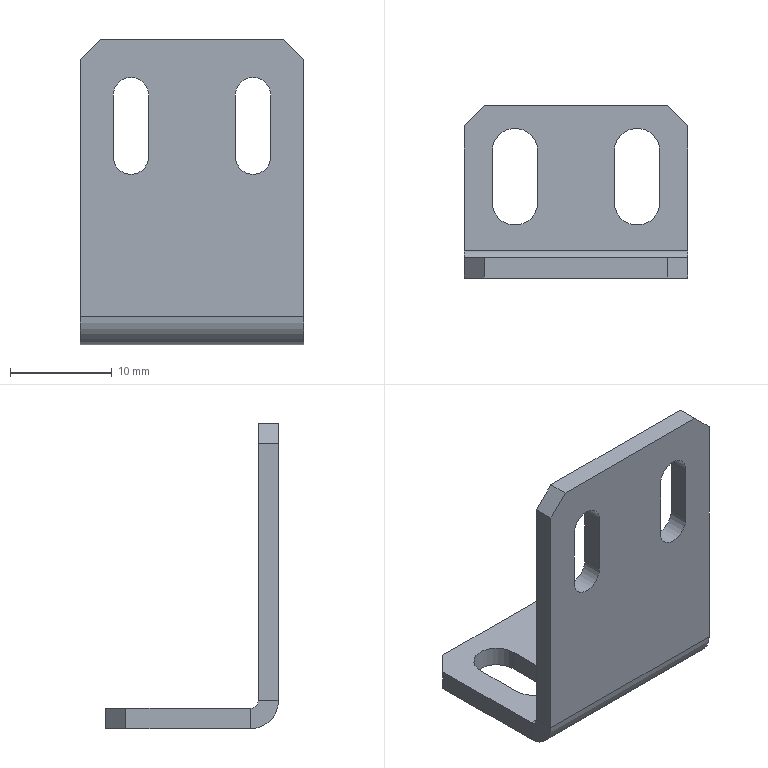Part | SolidWorks | features ICE 2, Chamfer 1, EdgeFlange 1, FlatPattern 1, SMBaseFlange 1, SheetMetal 1 | 1 solid | 36 faces | box 22 x 17 x 30 mm | volume 1655 mm3 | plane 24 | cylinder 12 | commonest cylinder face diameters 3.5 x6 4.5 x4 1.473 x1 5.473 x1
STEP:
#1=CARTESIAN_POINT('',(-6.,-2.,26.25));
#2=VERTEX_POINT('',#1);
#3=CARTESIAN_POINT('',(-4.25,-2.,24.5));
#4=VERTEX_POINT('',#3);
#5=CARTESIAN_POINT('',(-6.,-2.,24.5));
#6=DIRECTION('',(0.,1.,0.));
#7=DIRECTION('',(0.,0.,1.));
#8=AXIS2_PLACEMENT_3D('',#5,#6,#7);
#9=CIRCLE('',#8,1.75);
#10=EDGE_CURVE('',#2,#4,#9,.T.);
#11=ORIENTED_EDGE('',*,*,#10,.F.);
#12=CARTESIAN_POINT('',(-6.,0.,26.25));
#13=VERTEX_POINT('',#12);
#14=CARTESIAN_POINT('',(-6.,-10.,26.25));
#15=DIRECTION('',(0.,1.,0.));
#16=VECTOR('',#15,1000.);
#17=LINE('',#14,#16);
#18=EDGE_CURVE('',#2,#13,#17,.T.);
#19=ORIENTED_EDGE('',*,*,#18,.T.);
#20=CARTESIAN_POINT('',(-4.25,0.,24.5));
#21=VERTEX_POINT('',#20);
#22=CARTESIAN_POINT('',(-6.,0.,24.5));
#23=DIRECTION('',(0.,1.,0.));
#24=DIRECTION('',(0.,0.,1.));
#25=AXIS2_PLACEMENT_3D('',#22,#23,#24);
#26=CIRCLE('',#25,1.75);
#27=EDGE_CURVE('',#13,#21,#26,.T.);
#28=ORIENTED_EDGE('',*,*,#27,.T.);
#29=CARTESIAN_POINT('',(-4.25,-10.,24.5));
#30=DIRECTION('',(0.,1.,0.));
#31=VECTOR('',#30,1000.);
#32=LINE('',#29,#31);
#33=EDGE_CURVE('',#4,#21,#32,.T.);
#34=ORIENTED_EDGE('',*,*,#33,.F.);
#35=EDGE_LOOP('',(#11,#19,#28,#34));
#36=FACE_OUTER_BOUND('',#35,.T.);
#37=CARTESIAN_POINT('',(-6.,-10.,24.5));
#38=DIRECTION('',(0.,1.,0.));
#39=DIRECTION('',(0.,0.,1.));
#40=AXIS2_PLACEMENT_3D('',#37,#38,#39);
#41=CYLINDRICAL_SURFACE('',#40,1.75);
#42=ADVANCED_FACE('',(#36),#41,.F.);
#43=CARTESIAN_POINT('',(6.,-2.,26.25));
#44=VERTEX_POINT('',#43);
#45=CARTESIAN_POINT('',(7.75,-2.,24.5));
#46=VERTEX_POINT('',#45);
#47=CARTESIAN_POINT('',(6.,-2.,24.5));
#48=DIRECTION('',(0.,1.,0.));
#49=DIRECTION('',(0.,0.,1.));
#50=AXIS2_PLACEMENT_3D('',#47,#48,#49);
#51=CIRCLE('',#50,1.75);
#52=EDGE_CURVE('',#44,#46,#51,.T.);
#53=ORIENTED_EDGE('',*,*,#52,.F.);
#54=CARTESIAN_POINT('',(6.,0.,26.25));
#55=VERTEX_POINT('',#54);
#56=CARTESIAN_POINT('',(6.,-10.,26.25));
#57=DIRECTION('',(0.,1.,0.));
#58=VECTOR('',#57,1000.);
#59=LINE('',#56,#58);
#60=EDGE_CURVE('',#44,#55,#59,.T.);
#61=ORIENTED_EDGE('',*,*,#60,.T.);
#62=CARTESIAN_POINT('',(7.75,0.,24.5));
#63=VERTEX_POINT('',#62);
#64=CARTESIAN_POINT('',(6.,0.,24.5));
#65=DIRECTION('',(0.,1.,0.));
#66=DIRECTION('',(0.,0.,1.));
#67=AXIS2_PLACEMENT_3D('',#64,#65,#66);
#68=CIRCLE('',#67,1.75);
#69=EDGE_CURVE('',#55,#63,#68,.T.);
#70=ORIENTED_EDGE('',*,*,#69,.T.);
#71=CARTESIAN_POINT('',(7.75,-10.,24.5));
#72=DIRECTION('',(0.,1.,0.));
#73=VECTOR('',#72,1000.);
#74=LINE('',#71,#73);
#75=EDGE_CURVE('',#46,#63,#74,.T.);
#76=ORIENTED_EDGE('',*,*,#75,.F.);
#77=EDGE_LOOP('',(#53,#61,#70,#76));
#78=FACE_OUTER_BOUND('',#77,.T.);
#79=CARTESIAN_POINT('',(6.,-10.,24.5));
#80=DIRECTION('',(0.,1.,0.));
#81=DIRECTION('',(0.,0.,1.));
#82=AXIS2_PLACEMENT_3D('',#79,#80,#81);
#83=CYLINDRICAL_SURFACE('',#82,1.75);
#84=ADVANCED_FACE('',(#78),#83,.F.);
#85=CARTESIAN_POINT('',(-4.25,-2.,18.5));
#86=VERTEX_POINT('',#85);
#87=CARTESIAN_POINT('',(-4.25,-2.,30.));
#88=DIRECTION('',(0.,0.,-1.));
#89=VECTOR('',#88,1000.);
#90=LINE('',#87,#89);
#91=EDGE_CURVE('',#4,#86,#90,.T.);
#92=ORIENTED_EDGE('',*,*,#91,.T.);
#93=CARTESIAN_POINT('',(-7.75,-2.,18.5));
#94=VERTEX_POINT('',#93);
#95=CARTESIAN_POINT('',(-6.,-2.,18.5));
#96=DIRECTION('',(0.,1.,0.));
#97=DIRECTION('',(0.,0.,1.));
#98=AXIS2_PLACEMENT_3D('',#95,#96,#97);
#99=CIRCLE('',#98,1.75);
#100=EDGE_CURVE('',#86,#94,#99,.T.);
#101=ORIENTED_EDGE('',*,*,#100,.T.);
#102=CARTESIAN_POINT('',(-7.75,-2.,24.5));
#103=VERTEX_POINT('',#102);
#104=CARTESIAN_POINT('',(-7.75,-2.,30.));
#105=DIRECTION('',(0.,0.,1.));
#106=VECTOR('',#105,1000.);
#107=LINE('',#104,#106);
#108=EDGE_CURVE('',#94,#103,#107,.T.);
#109=ORIENTED_EDGE('',*,*,#108,.T.);
#110=CARTESIAN_POINT('',(-6.,-2.,24.5));
#111=DIRECTION('',(0.,1.,0.));
#112=DIRECTION('',(0.,0.,1.));
#113=AXIS2_PLACEMENT_3D('',#110,#111,#112);
#114=CIRCLE('',#113,1.75);
#115=EDGE_CURVE('',#103,#2,#114,.T.);
#116=ORIENTED_EDGE('',*,*,#115,.T.);
#117=ORIENTED_EDGE('',*,*,#10,.T.);
#118=EDGE_LOOP('',(#92,#101,#109,#116,#117));
#119=FACE_BOUND('',#118,.T.);
#120=CARTESIAN_POINT('',(7.75,-2.,18.5));
#121=VERTEX_POINT('',#120);
#122=CARTESIAN_POINT('',(7.75,-2.,30.));
#123=DIRECTION('',(0.,0.,-1.));
#124=VECTOR('',#123,1000.);
#125=LINE('',#122,#124);
#126=EDGE_CURVE('',#46,#121,#125,.T.);
#127=ORIENTED_EDGE('',*,*,#126,.T.);
#128=CARTESIAN_POINT('',(4.25,-2.,18.5));
#129=VERTEX_POINT('',#128);
#130=CARTESIAN_POINT('',(6.,-2.,18.5));
#131=DIRECTION('',(0.,1.,0.));
#132=DIRECTION('',(0.,0.,1.));
#133=AXIS2_PLACEMENT_3D('',#130,#131,#132);
#134=CIRCLE('',#133,1.75);
#135=EDGE_CURVE('',#121,#129,#134,.T.);
#136=ORIENTED_EDGE('',*,*,#135,.T.);
#137=CARTESIAN_POINT('',(4.25,-2.,24.5));
#138=VERTEX_POINT('',#137);
#139=CARTESIAN_POINT('',(4.25,-2.,30.));
#140=DIRECTION('',(0.,0.,1.));
#141=VECTOR('',#140,1000.);
#142=LINE('',#139,#141);
#143=EDGE_CURVE('',#129,#138,#142,.T.);
#144=ORIENTED_EDGE('',*,*,#143,.T.);
#145=CARTESIAN_POINT('',(6.,-2.,24.5));
#146=DIRECTION('',(0.,1.,0.));
#147=DIRECTION('',(0.,0.,1.));
#148=AXIS2_PLACEMENT_3D('',#145,#146,#147);
#149=CIRCLE('',#148,1.75);
#150=EDGE_CURVE('',#138,#44,#149,.T.);
#151=ORIENTED_EDGE('',*,*,#150,.T.);
#152=ORIENTED_EDGE('',*,*,#52,.T.);
#153=EDGE_LOOP('',(#127,#136,#144,#151,#152));
#154=FACE_BOUND('',#153,.T.);
#155=CARTESIAN_POINT('',(-9.,-2.,30.));
#156=VERTEX_POINT('',#155);
#157=CARTESIAN_POINT('',(9.,-2.,30.));
#158=VERTEX_POINT('',#157);
#159=CARTESIAN_POINT('',(-11.,-2.,30.));
#160=DIRECTION('',(1.,0.,0.));
#161=VECTOR('',#160,1000.);
#162=LINE('',#159,#161);
#163=EDGE_CURVE('',#156,#158,#162,.T.);
#164=ORIENTED_EDGE('',*,*,#163,.F.);
#165=CARTESIAN_POINT('',(-11.,-2.,28.));
#166=VERTEX_POINT('',#165);
#167=CARTESIAN_POINT('',(-11.,-2.,28.));
#168=DIRECTION('',(-0.7071,0.,-0.7071));
#169=VECTOR('',#168,1000.);
#170=LINE('',#167,#169);
#171=EDGE_CURVE('',#156,#166,#170,.T.);
#172=ORIENTED_EDGE('',*,*,#171,.T.);
#173=CARTESIAN_POINT('',(-11.,-2.,2.737));
#174=VERTEX_POINT('',#173);
#175=CARTESIAN_POINT('',(-11.,-2.,30.));
#176=DIRECTION('',(0.,0.,-1.));
#177=VECTOR('',#176,1000.);
#178=LINE('',#175,#177);
#179=EDGE_CURVE('',#166,#174,#178,.T.);
#180=ORIENTED_EDGE('',*,*,#179,.T.);
#181=CARTESIAN_POINT('',(11.,-2.,2.737));
#182=VERTEX_POINT('',#181);
#183=CARTESIAN_POINT('',(-11.,-2.,2.737));
#184=DIRECTION('',(1.,0.,0.));
#185=VECTOR('',#184,1000.);
#186=LINE('',#183,#185);
#187=EDGE_CURVE('',#174,#182,#186,.T.);
#188=ORIENTED_EDGE('',*,*,#187,.T.);
#189=CARTESIAN_POINT('',(11.,-2.,28.));
#190=VERTEX_POINT('',#189);
#191=CARTESIAN_POINT('',(11.,-2.,30.));
#192=DIRECTION('',(0.,0.,-1.));
#193=VECTOR('',#192,1000.);
#194=LINE('',#191,#193);
#195=EDGE_CURVE('',#190,#182,#194,.T.);
#196=ORIENTED_EDGE('',*,*,#195,.F.);
#197=CARTESIAN_POINT('',(11.,-2.,28.));
#198=DIRECTION('',(-0.7071,0.,0.7071));
#199=VECTOR('',#198,1000.);
#200=LINE('',#197,#199);
#201=EDGE_CURVE('',#190,#158,#200,.T.);
#202=ORIENTED_EDGE('',*,*,#201,.T.);
#203=EDGE_LOOP('',(#164,#172,#180,#188,#196,#202));
#204=FACE_OUTER_BOUND('',#203,.T.);
#205=CARTESIAN_POINT('',(-11.,-2.,30.));
#206=DIRECTION('',(0.,1.,0.));
#207=DIRECTION('',(0.,0.,1.));
#208=AXIS2_PLACEMENT_3D('',#205,#206,#207);
#209=PLANE('',#208);
#210=ADVANCED_FACE('',(#119,#154,#204),#209,.F.);
#211=CARTESIAN_POINT('',(-4.25,0.,18.5));
#212=VERTEX_POINT('',#211);
#213=CARTESIAN_POINT('',(-7.75,0.,18.5));
#214=VERTEX_POINT('',#213);
#215=CARTESIAN_POINT('',(-6.,0.,18.5));
#216=DIRECTION('',(0.,1.,0.));
#217=DIRECTION('',(0.,0.,1.));
#218=AXIS2_PLACEMENT_3D('',#215,#216,#217);
#219=CIRCLE('',#218,1.75);
#220=EDGE_CURVE('',#212,#214,#219,.T.);
#221=ORIENTED_EDGE('',*,*,#220,.F.);
#222=CARTESIAN_POINT('',(-4.25,0.,18.5));
#223=DIRECTION('',(0.,0.,-1.));
#224=VECTOR('',#223,1000.);
#225=LINE('',#222,#224);
#226=EDGE_CURVE('',#21,#212,#225,.T.);
#227=ORIENTED_EDGE('',*,*,#226,.F.);
#228=ORIENTED_EDGE('',*,*,#27,.F.);
#229=CARTESIAN_POINT('',(-7.75,0.,24.5));
#230=VERTEX_POINT('',#229);
#231=CARTESIAN_POINT('',(-6.,0.,24.5));
#232=DIRECTION('',(0.,1.,0.));
#233=DIRECTION('',(0.,0.,1.));
#234=AXIS2_PLACEMENT_3D('',#231,#232,#233);
#235=CIRCLE('',#234,1.75);
#236=EDGE_CURVE('',#230,#13,#235,.T.);
#237=ORIENTED_EDGE('',*,*,#236,.F.);
#238=CARTESIAN_POINT('',(-7.75,0.,18.5));
#239=DIRECTION('',(0.,0.,1.));
#240=VECTOR('',#239,1000.);
#241=LINE('',#238,#240);
#242=EDGE_CURVE('',#214,#230,#241,.T.);
#243=ORIENTED_EDGE('',*,*,#242,.F.);
#244=EDGE_LOOP('',(#221,#227,#228,#237,#243));
#245=FACE_BOUND('',#244,.T.);
#246=CARTESIAN_POINT('',(7.75,0.,18.5));
#247=VERTEX_POINT('',#246);
#248=CARTESIAN_POINT('',(4.25,0.,18.5));
#249=VERTEX_POINT('',#248);
#250=CARTESIAN_POINT('',(6.,0.,18.5));
#251=DIRECTION('',(0.,1.,0.));
#252=DIRECTION('',(0.,0.,1.));
#253=AXIS2_PLACEMENT_3D('',#250,#251,#252);
#254=CIRCLE('',#253,1.75);
#255=EDGE_CURVE('',#247,#249,#254,.T.);
#256=ORIENTED_EDGE('',*,*,#255,.F.);
#257=CARTESIAN_POINT('',(7.75,0.,18.5));
#258=DIRECTION('',(0.,0.,-1.));
#259=VECTOR('',#258,1000.);
#260=LINE('',#257,#259);
#261=EDGE_CURVE('',#63,#247,#260,.T.);
#262=ORIENTED_EDGE('',*,*,#261,.F.);
#263=ORIENTED_EDGE('',*,*,#69,.F.);
#264=CARTESIAN_POINT('',(4.25,0.,24.5));
#265=VERTEX_POINT('',#264);
#266=CARTESIAN_POINT('',(6.,0.,24.5));
#267=DIRECTION('',(0.,1.,0.));
#268=DIRECTION('',(0.,0.,1.));
#269=AXIS2_PLACEMENT_3D('',#266,#267,#268);
#270=CIRCLE('',#269,1.75);
#271=EDGE_CURVE('',#265,#55,#270,.T.);
#272=ORIENTED_EDGE('',*,*,#271,.F.);
#273=CARTESIAN_POINT('',(4.25,0.,18.5));
#274=DIRECTION('',(0.,0.,1.));
#275=VECTOR('',#274,1000.);
#276=LINE('',#273,#275);
#277=EDGE_CURVE('',#249,#265,#276,.T.);
#278=ORIENTED_EDGE('',*,*,#277,.F.);
#279=EDGE_LOOP('',(#256,#262,#263,#272,#278));
#280=FACE_BOUND('',#279,.T.);
#281=CARTESIAN_POINT('',(-11.,0.,28.));
#282=VERTEX_POINT('',#281);
#283=CARTESIAN_POINT('',(-11.,0.,2.737));
#284=VERTEX_POINT('',#283);
#285=CARTESIAN_POINT('',(-11.,0.,30.));
#286=DIRECTION('',(0.,0.,-1.));
#287=VECTOR('',#286,1000.);
#288=LINE('',#285,#287);
#289=EDGE_CURVE('',#282,#284,#288,.T.);
#290=ORIENTED_EDGE('',*,*,#289,.F.);
#291=CARTESIAN_POINT('',(-9.,0.,30.));
#292=VERTEX_POINT('',#291);
#293=CARTESIAN_POINT('',(-10.,0.,29.));
#294=DIRECTION('',(0.7071,0.,0.7071));
#295=VECTOR('',#294,1000.);
#296=LINE('',#293,#295);
#297=EDGE_CURVE('',#282,#292,#296,.T.);
#298=ORIENTED_EDGE('',*,*,#297,.T.);
#299=CARTESIAN_POINT('',(9.,0.,30.));
#300=VERTEX_POINT('',#299);
#301=CARTESIAN_POINT('',(-11.,0.,30.));
#302=DIRECTION('',(1.,0.,0.));
#303=VECTOR('',#302,1000.);
#304=LINE('',#301,#303);
#305=EDGE_CURVE('',#292,#300,#304,.T.);
#306=ORIENTED_EDGE('',*,*,#305,.T.);
#307=CARTESIAN_POINT('',(11.,0.,28.));
#308=VERTEX_POINT('',#307);
#309=CARTESIAN_POINT('',(-1.,0.,40.));
#310=DIRECTION('',(0.7071,0.,-0.7071));
#311=VECTOR('',#310,1000.);
#312=LINE('',#309,#311);
#313=EDGE_CURVE('',#300,#308,#312,.T.);
#314=ORIENTED_EDGE('',*,*,#313,.T.);
#315=CARTESIAN_POINT('',(11.,0.,2.737));
#316=VERTEX_POINT('',#315);
#317=CARTESIAN_POINT('',(11.,0.,30.));
#318=DIRECTION('',(0.,0.,-1.));
#319=VECTOR('',#318,1000.);
#320=LINE('',#317,#319);
#321=EDGE_CURVE('',#308,#316,#320,.T.);
#322=ORIENTED_EDGE('',*,*,#321,.T.);
#323=CARTESIAN_POINT('',(-11.,0.,2.737));
#324=DIRECTION('',(1.,0.,0.));
#325=VECTOR('',#324,1000.);
#326=LINE('',#323,#325);
#327=EDGE_CURVE('',#284,#316,#326,.T.);
#328=ORIENTED_EDGE('',*,*,#327,.F.);
#329=EDGE_LOOP('',(#290,#298,#306,#314,#322,#328));
#330=FACE_OUTER_BOUND('',#329,.T.);
#331=CARTESIAN_POINT('',(-11.,0.,30.));
#332=DIRECTION('',(0.,1.,0.));
#333=DIRECTION('',(0.,0.,1.));
#334=AXIS2_PLACEMENT_3D('',#331,#332,#333);
#335=PLANE('',#334);
#336=ADVANCED_FACE('',(#245,#280,#330),#335,.T.);
#337=ORIENTED_EDGE('',*,*,#179,.F.);
#338=CARTESIAN_POINT('',(-11.,0.,28.));
#339=DIRECTION('',(0.,1.,0.));
#340=VECTOR('',#339,1000.);
#341=LINE('',#338,#340);
#342=EDGE_CURVE('',#166,#282,#341,.T.);
#343=ORIENTED_EDGE('',*,*,#342,.T.);
#344=ORIENTED_EDGE('',*,*,#289,.T.);
#345=CARTESIAN_POINT('',(-11.,0.,2.737));
#346=DIRECTION('',(0.,-1.,0.));
#347=VECTOR('',#346,1000.);
#348=LINE('',#345,#347);
#349=EDGE_CURVE('',#284,#174,#348,.T.);
#350=ORIENTED_EDGE('',*,*,#349,.T.);
#351=EDGE_LOOP('',(#337,#343,#344,#350));
#352=FACE_OUTER_BOUND('',#351,.T.);
#353=CARTESIAN_POINT('',(-11.,-2.,30.));
#354=DIRECTION('',(-1.,0.,0.));
#355=DIRECTION('',(0.,0.,1.));
#356=AXIS2_PLACEMENT_3D('',#353,#354,#355);
#357=PLANE('',#356);
#358=ADVANCED_FACE('',(#352),#357,.T.);
#359=ORIENTED_EDGE('',*,*,#321,.F.);
#360=CARTESIAN_POINT('',(11.,-2.,28.));
#361=DIRECTION('',(0.,-1.,0.));
#362=VECTOR('',#361,1000.);
#363=LINE('',#360,#362);
#364=EDGE_CURVE('',#308,#190,#363,.T.);
#365=ORIENTED_EDGE('',*,*,#364,.T.);
#366=ORIENTED_EDGE('',*,*,#195,.T.);
#367=CARTESIAN_POINT('',(11.,0.,2.737));
#368=DIRECTION('',(0.,-1.,0.));
#369=VECTOR('',#368,1000.);
#370=LINE('',#367,#369);
#371=EDGE_CURVE('',#316,#182,#370,.T.);
#372=ORIENTED_EDGE('',*,*,#371,.F.);
#373=EDGE_LOOP('',(#359,#365,#366,#372));
#374=FACE_OUTER_BOUND('',#373,.T.);
#375=CARTESIAN_POINT('',(11.,0.,30.));
#376=DIRECTION('',(1.,0.,0.));
#377=DIRECTION('',(0.,0.,-1.));
#378=AXIS2_PLACEMENT_3D('',#375,#376,#377);
#379=PLANE('',#378);
#380=ADVANCED_FACE('',(#374),#379,.T.);
#381=ORIENTED_EDGE('',*,*,#305,.F.);
#382=CARTESIAN_POINT('',(-9.,-2.,30.));
#383=DIRECTION('',(0.,-1.,0.));
#384=VECTOR('',#383,1000.);
#385=LINE('',#382,#384);
#386=EDGE_CURVE('',#292,#156,#385,.T.);
#387=ORIENTED_EDGE('',*,*,#386,.T.);
#388=ORIENTED_EDGE('',*,*,#163,.T.);
#389=CARTESIAN_POINT('',(9.,0.,30.));
#390=DIRECTION('',(0.,1.,0.));
#391=VECTOR('',#390,1000.);
#392=LINE('',#389,#391);
#393=EDGE_CURVE('',#158,#300,#392,.T.);
#394=ORIENTED_EDGE('',*,*,#393,.T.);
#395=EDGE_LOOP('',(#381,#387,#388,#394));
#396=FACE_OUTER_BOUND('',#395,.T.);
#397=CARTESIAN_POINT('',(0.,0.,30.));
#398=DIRECTION('',(0.,0.,-1.));
#399=DIRECTION('',(-1.,0.,0.));
#400=AXIS2_PLACEMENT_3D('',#397,#398,#399);
#401=PLANE('',#400);
#402=ADVANCED_FACE('',(#396),#401,.F.);
#403=CARTESIAN_POINT('',(11.,0.7366,2.));
#404=VERTEX_POINT('',#403);
#405=CARTESIAN_POINT('',(11.,0.7366,0.));
#406=VERTEX_POINT('',#405);
#407=CARTESIAN_POINT('',(11.,0.7366,0.));
#408=DIRECTION('',(0.,0.,-1.));
#409=VECTOR('',#408,1000.);
#410=LINE('',#407,#409);
#411=EDGE_CURVE('',#404,#406,#410,.T.);
#412=ORIENTED_EDGE('',*,*,#411,.F.);
#413=CARTESIAN_POINT('',(11.,0.7366,2.737));
#414=DIRECTION('',(1.,0.,0.));
#415=DIRECTION('',(0.,0.,1.));
#416=AXIS2_PLACEMENT_3D('',#413,#414,#415);
#417=CIRCLE('',#416,0.7366);
#418=EDGE_CURVE('',#316,#404,#417,.T.);
#419=ORIENTED_EDGE('',*,*,#418,.F.);
#420=ORIENTED_EDGE('',*,*,#371,.T.);
#421=CARTESIAN_POINT('',(11.,0.7366,2.737));
#422=DIRECTION('',(1.,0.,0.));
#423=DIRECTION('',(0.,0.,1.));
#424=AXIS2_PLACEMENT_3D('',#421,#422,#423);
#425=CIRCLE('',#424,2.737);
#426=EDGE_CURVE('',#182,#406,#425,.T.);
#427=ORIENTED_EDGE('',*,*,#426,.T.);
#428=EDGE_LOOP('',(#412,#419,#420,#427));
#429=FACE_OUTER_BOUND('',#428,.T.);
#430=CARTESIAN_POINT('',(11.,0.7366,2.737));
#431=DIRECTION('',(1.,0.,0.));
#432=DIRECTION('',(0.,0.,-1.));
#433=AXIS2_PLACEMENT_3D('',#430,#431,#432);
#434=PLANE('',#433);
#435=ADVANCED_FACE('',(#429),#434,.T.);
#436=CARTESIAN_POINT('',(-11.,0.7366,2.));
#437=VERTEX_POINT('',#436);
#438=CARTESIAN_POINT('',(-11.,0.7366,2.737));
#439=DIRECTION('',(-1.,0.,0.));
#440=DIRECTION('',(0.,0.,1.));
#441=AXIS2_PLACEMENT_3D('',#438,#439,#440);
#442=CIRCLE('',#441,0.7366);
#443=EDGE_CURVE('',#437,#284,#442,.T.);
#444=ORIENTED_EDGE('',*,*,#443,.F.);
#445=CARTESIAN_POINT('',(-11.,0.7366,0.));
#446=VERTEX_POINT('',#445);
#447=CARTESIAN_POINT('',(-11.,0.7366,2.));
#448=DIRECTION('',(0.,0.,-1.));
#449=VECTOR('',#448,1000.);
#450=LINE('',#447,#449);
#451=EDGE_CURVE('',#437,#446,#450,.T.);
#452=ORIENTED_EDGE('',*,*,#451,.T.);
#453=CARTESIAN_POINT('',(-11.,0.7366,2.737));
#454=DIRECTION('',(-1.,0.,0.));
#455=DIRECTION('',(0.,0.,1.));
#456=AXIS2_PLACEMENT_3D('',#453,#454,#455);
#457=CIRCLE('',#456,2.737);
#458=EDGE_CURVE('',#446,#174,#457,.T.);
#459=ORIENTED_EDGE('',*,*,#458,.T.);
#460=ORIENTED_EDGE('',*,*,#349,.F.);
#461=EDGE_LOOP('',(#444,#452,#459,#460));
#462=FACE_OUTER_BOUND('',#461,.T.);
#463=CARTESIAN_POINT('',(-11.,0.7366,2.737));
#464=DIRECTION('',(1.,0.,0.));
#465=DIRECTION('',(0.,0.,-1.));
#466=AXIS2_PLACEMENT_3D('',#463,#464,#465);
#467=PLANE('',#466);
#468=ADVANCED_FACE('',(#462),#467,.F.);
#469=ORIENTED_EDGE('',*,*,#187,.F.);
#470=ORIENTED_EDGE('',*,*,#458,.F.);
#471=CARTESIAN_POINT('',(11.,0.7366,0.));
#472=DIRECTION('',(1.,0.,0.));
#473=VECTOR('',#472,1000.);
#474=LINE('',#471,#473);
#475=EDGE_CURVE('',#446,#406,#474,.T.);
#476=ORIENTED_EDGE('',*,*,#475,.T.);
#477=ORIENTED_EDGE('',*,*,#426,.F.);
#478=EDGE_LOOP('',(#469,#470,#476,#477));
#479=FACE_OUTER_BOUND('',#478,.T.);
#480=CARTESIAN_POINT('',(-11.,0.7366,2.737));
#481=DIRECTION('',(-1.,0.,0.));
#482=DIRECTION('',(0.,0.,-1.));
#483=AXIS2_PLACEMENT_3D('',#480,#481,#482);
#484=CYLINDRICAL_SURFACE('',#483,2.737);
#485=ADVANCED_FACE('',(#479),#484,.T.);
#486=ORIENTED_EDGE('',*,*,#327,.T.);
#487=ORIENTED_EDGE('',*,*,#418,.T.);
#488=CARTESIAN_POINT('',(11.,0.7366,2.));
#489=DIRECTION('',(-1.,0.,0.));
#490=VECTOR('',#489,1000.);
#491=LINE('',#488,#490);
#492=EDGE_CURVE('',#404,#437,#491,.T.);
#493=ORIENTED_EDGE('',*,*,#492,.T.);
#494=ORIENTED_EDGE('',*,*,#443,.T.);
#495=EDGE_LOOP('',(#486,#487,#493,#494));
#496=FACE_OUTER_BOUND('',#495,.T.);
#497=CARTESIAN_POINT('',(-11.,0.7366,2.737));
#498=DIRECTION('',(-1.,0.,0.));
#499=DIRECTION('',(0.,0.,-1.));
#500=AXIS2_PLACEMENT_3D('',#497,#498,#499);
#501=CYLINDRICAL_SURFACE('',#500,0.7366);
#502=ADVANCED_FACE('',(#496),#501,.F.);
#503=CARTESIAN_POINT('',(-11.,13.,2.));
#504=VERTEX_POINT('',#503);
#505=CARTESIAN_POINT('',(-11.,15.,2.));
#506=DIRECTION('',(0.,1.,0.));
#507=VECTOR('',#506,1000.);
#508=LINE('',#505,#507);
#509=EDGE_CURVE('',#437,#504,#508,.T.);
#510=ORIENTED_EDGE('',*,*,#509,.T.);
#511=CARTESIAN_POINT('',(-11.,13.,0.));
#512=VERTEX_POINT('',#511);
#513=CARTESIAN_POINT('',(-11.,13.,0.));
#514=DIRECTION('',(0.,0.,-1.));
#515=VECTOR('',#514,1000.);
#516=LINE('',#513,#515);
#517=EDGE_CURVE('',#504,#512,#516,.T.);
#518=ORIENTED_EDGE('',*,*,#517,.T.);
#519=CARTESIAN_POINT('',(-11.,0.,0.));
#520=DIRECTION('',(0.,1.,0.));
#521=VECTOR('',#520,1000.);
#522=LINE('',#519,#521);
#523=EDGE_CURVE('',#446,#512,#522,.T.);
#524=ORIENTED_EDGE('',*,*,#523,.F.);
#525=ORIENTED_EDGE('',*,*,#451,.F.);
#526=EDGE_LOOP('',(#510,#518,#524,#525));
#527=FACE_OUTER_BOUND('',#526,.T.);
#528=CARTESIAN_POINT('',(-11.,15.,0.));
#529=DIRECTION('',(1.,0.,0.));
#530=DIRECTION('',(0.,1.,0.));
#531=AXIS2_PLACEMENT_3D('',#528,#529,#530);
#532=PLANE('',#531);
#533=ADVANCED_FACE('',(#527),#532,.F.);
#534=CARTESIAN_POINT('',(11.,13.,0.));
#535=VERTEX_POINT('',#534);
#536=CARTESIAN_POINT('',(11.,0.,0.));
#537=DIRECTION('',(0.,-1.,0.));
#538=VECTOR('',#537,1000.);
#539=LINE('',#536,#538);
#540=EDGE_CURVE('',#535,#406,#539,.T.);
#541=ORIENTED_EDGE('',*,*,#540,.F.);
#542=CARTESIAN_POINT('',(11.,13.,2.));
#543=VERTEX_POINT('',#542);
#544=CARTESIAN_POINT('',(11.,13.,0.));
#545=DIRECTION('',(0.,0.,1.));
#546=VECTOR('',#545,1000.);
#547=LINE('',#544,#546);
#548=EDGE_CURVE('',#535,#543,#547,.T.);
#549=ORIENTED_EDGE('',*,*,#548,.T.);
#550=CARTESIAN_POINT('',(11.,0.,2.));
#551=DIRECTION('',(0.,-1.,0.));
#552=VECTOR('',#551,1000.);
#553=LINE('',#550,#552);
#554=EDGE_CURVE('',#543,#404,#553,.T.);
#555=ORIENTED_EDGE('',*,*,#554,.T.);
#556=ORIENTED_EDGE('',*,*,#411,.T.);
#557=EDGE_LOOP('',(#541,#549,#555,#556));
#558=FACE_OUTER_BOUND('',#557,.T.);
#559=CARTESIAN_POINT('',(11.,0.,0.));
#560=DIRECTION('',(-1.,0.,0.));
#561=DIRECTION('',(0.,0.,1.));
#562=AXIS2_PLACEMENT_3D('',#559,#560,#561);
#563=PLANE('',#562);
#564=ADVANCED_FACE('',(#558),#563,.F.);
#565=CARTESIAN_POINT('',(-3.75,5.5,0.));
#566=VERTEX_POINT('',#565);
#567=CARTESIAN_POINT('',(-3.75,10.5,0.));
#568=VERTEX_POINT('',#567);
#569=CARTESIAN_POINT('',(-3.75,0.,0.));
#570=DIRECTION('',(0.,1.,0.));
#571=VECTOR('',#570,1000.);
#572=LINE('',#569,#571);
#573=EDGE_CURVE('',#566,#568,#572,.T.);
#574=ORIENTED_EDGE('',*,*,#573,.T.);
#575=CARTESIAN_POINT('',(-8.25,10.5,0.));
#576=VERTEX_POINT('',#575);
#577=CARTESIAN_POINT('',(-6.,10.5,0.));
#578=DIRECTION('',(0.,0.,1.));
#579=DIRECTION('',(0.,-1.,0.));
#580=AXIS2_PLACEMENT_3D('',#577,#578,#579);
#581=CIRCLE('',#580,2.25);
#582=EDGE_CURVE('',#568,#576,#581,.T.);
#583=ORIENTED_EDGE('',*,*,#582,.T.);
#584=CARTESIAN_POINT('',(-8.25,5.5,0.));
#585=VERTEX_POINT('',#584);
#586=CARTESIAN_POINT('',(-8.25,0.,0.));
#587=DIRECTION('',(0.,-1.,0.));
#588=VECTOR('',#587,1000.);
#589=LINE('',#586,#588);
#590=EDGE_CURVE('',#576,#585,#589,.T.);
#591=ORIENTED_EDGE('',*,*,#590,.T.);
#592=CARTESIAN_POINT('',(-6.,5.5,0.));
#593=DIRECTION('',(0.,0.,1.));
#594=DIRECTION('',(0.,-1.,0.));
#595=AXIS2_PLACEMENT_3D('',#592,#593,#594);
#596=CIRCLE('',#595,2.25);
#597=EDGE_CURVE('',#585,#566,#596,.T.);
#598=ORIENTED_EDGE('',*,*,#597,.T.);
#599=EDGE_LOOP('',(#574,#583,#591,#598));
#600=FACE_BOUND('',#599,.T.);
#601=CARTESIAN_POINT('',(8.25,5.5,0.));
#602=VERTEX_POINT('',#601);
#603=CARTESIAN_POINT('',(8.25,10.5,0.));
#604=VERTEX_POINT('',#603);
#605=CARTESIAN_POINT('',(8.25,0.,0.));
#606=DIRECTION('',(0.,1.,0.));
#607=VECTOR('',#606,1000.);
#608=LINE('',#605,#607);
#609=EDGE_CURVE('',#602,#604,#608,.T.);
#610=ORIENTED_EDGE('',*,*,#609,.T.);
#611=CARTESIAN_POINT('',(3.75,10.5,0.));
#612=VERTEX_POINT('',#611);
#613=CARTESIAN_POINT('',(6.,10.5,0.));
#614=DIRECTION('',(0.,0.,1.));
#615=DIRECTION('',(0.,-1.,0.));
#616=AXIS2_PLACEMENT_3D('',#613,#614,#615);
#617=CIRCLE('',#616,2.25);
#618=EDGE_CURVE('',#604,#612,#617,.T.);
#619=ORIENTED_EDGE('',*,*,#618,.T.);
#620=CARTESIAN_POINT('',(3.75,5.5,0.));
#621=VERTEX_POINT('',#620);
#622=CARTESIAN_POINT('',(3.75,0.,0.));
#623=DIRECTION('',(0.,-1.,0.));
#624=VECTOR('',#623,1000.);
#625=LINE('',#622,#624);
#626=EDGE_CURVE('',#612,#621,#625,.T.);
#627=ORIENTED_EDGE('',*,*,#626,.T.);
#628=CARTESIAN_POINT('',(6.,5.5,0.));
#629=DIRECTION('',(0.,0.,1.));
#630=DIRECTION('',(0.,-1.,0.));
#631=AXIS2_PLACEMENT_3D('',#628,#629,#630);
#632=CIRCLE('',#631,2.25);
#633=EDGE_CURVE('',#621,#602,#632,.T.);
#634=ORIENTED_EDGE('',*,*,#633,.T.);
#635=EDGE_LOOP('',(#610,#619,#627,#634));
#636=FACE_BOUND('',#635,.T.);
#637=ORIENTED_EDGE('',*,*,#523,.T.);
#638=CARTESIAN_POINT('',(-9.,15.,0.));
#639=VERTEX_POINT('',#638);
#640=CARTESIAN_POINT('',(-9.,15.,0.));
#641=DIRECTION('',(0.7071,0.7071,0.));
#642=VECTOR('',#641,1000.);
#643=LINE('',#640,#642);
#644=EDGE_CURVE('',#512,#639,#643,.T.);
#645=ORIENTED_EDGE('',*,*,#644,.T.);
#646=CARTESIAN_POINT('',(9.,15.,0.));
#647=VERTEX_POINT('',#646);
#648=CARTESIAN_POINT('',(0.,15.,0.));
#649=DIRECTION('',(1.,0.,0.));
#650=VECTOR('',#649,1000.);
#651=LINE('',#648,#650);
#652=EDGE_CURVE('',#639,#647,#651,.T.);
#653=ORIENTED_EDGE('',*,*,#652,.T.);
#654=CARTESIAN_POINT('',(11.,13.,0.));
#655=DIRECTION('',(0.7071,-0.7071,0.));
#656=VECTOR('',#655,1000.);
#657=LINE('',#654,#656);
#658=EDGE_CURVE('',#647,#535,#657,.T.);
#659=ORIENTED_EDGE('',*,*,#658,.T.);
#660=ORIENTED_EDGE('',*,*,#540,.T.);
#661=ORIENTED_EDGE('',*,*,#475,.F.);
#662=EDGE_LOOP('',(#637,#645,#653,#659,#660,#661));
#663=FACE_OUTER_BOUND('',#662,.T.);
#664=CARTESIAN_POINT('',(0.,0.,0.));
#665=DIRECTION('',(0.,0.,1.));
#666=DIRECTION('',(0.,-1.,0.));
#667=AXIS2_PLACEMENT_3D('',#664,#665,#666);
#668=PLANE('',#667);
#669=ADVANCED_FACE('',(#600,#636,#663),#668,.F.);
#670=CARTESIAN_POINT('',(-3.75,10.5,2.));
#671=VERTEX_POINT('',#670);
#672=CARTESIAN_POINT('',(-8.25,10.5,2.));
#673=VERTEX_POINT('',#672);
#674=CARTESIAN_POINT('',(-6.,10.5,2.));
#675=DIRECTION('',(0.,0.,1.));
#676=DIRECTION('',(1.,0.,0.));
#677=AXIS2_PLACEMENT_3D('',#674,#675,#676);
#678=CIRCLE('',#677,2.25);
#679=EDGE_CURVE('',#671,#673,#678,.T.);
#680=ORIENTED_EDGE('',*,*,#679,.F.);
#681=CARTESIAN_POINT('',(-3.75,5.5,2.));
#682=VERTEX_POINT('',#681);
#683=CARTESIAN_POINT('',(-3.75,10.5,2.));
#684=DIRECTION('',(0.,1.,0.));
#685=VECTOR('',#684,1000.);
#686=LINE('',#683,#685);
#687=EDGE_CURVE('',#682,#671,#686,.T.);
#688=ORIENTED_EDGE('',*,*,#687,.F.);
#689=CARTESIAN_POINT('',(-8.25,5.5,2.));
#690=VERTEX_POINT('',#689);
#691=CARTESIAN_POINT('',(-6.,5.5,2.));
#692=DIRECTION('',(0.,0.,1.));
#693=DIRECTION('',(1.,0.,0.));
#694=AXIS2_PLACEMENT_3D('',#691,#692,#693);
#695=CIRCLE('',#694,2.25);
#696=EDGE_CURVE('',#690,#682,#695,.T.);
#697=ORIENTED_EDGE('',*,*,#696,.F.);
#698=CARTESIAN_POINT('',(-8.25,10.5,2.));
#699=DIRECTION('',(0.,-1.,0.));
#700=VECTOR('',#699,1000.);
#701=LINE('',#698,#700);
#702=EDGE_CURVE('',#673,#690,#701,.T.);
#703=ORIENTED_EDGE('',*,*,#702,.F.);
#704=EDGE_LOOP('',(#680,#688,#697,#703));
#705=FACE_BOUND('',#704,.T.);
#706=CARTESIAN_POINT('',(8.25,10.5,2.));
#707=VERTEX_POINT('',#706);
#708=CARTESIAN_POINT('',(3.75,10.5,2.));
#709=VERTEX_POINT('',#708);
#710=CARTESIAN_POINT('',(6.,10.5,2.));
#711=DIRECTION('',(0.,0.,1.));
#712=DIRECTION('',(1.,0.,0.));
#713=AXIS2_PLACEMENT_3D('',#710,#711,#712);
#714=CIRCLE('',#713,2.25);
#715=EDGE_CURVE('',#707,#709,#714,.T.);
#716=ORIENTED_EDGE('',*,*,#715,.F.);
#717=CARTESIAN_POINT('',(8.25,5.5,2.));
#718=VERTEX_POINT('',#717);
#719=CARTESIAN_POINT('',(8.25,10.5,2.));
#720=DIRECTION('',(0.,1.,0.));
#721=VECTOR('',#720,1000.);
#722=LINE('',#719,#721);
#723=EDGE_CURVE('',#718,#707,#722,.T.);
#724=ORIENTED_EDGE('',*,*,#723,.F.);
#725=CARTESIAN_POINT('',(3.75,5.5,2.));
#726=VERTEX_POINT('',#725);
#727=CARTESIAN_POINT('',(6.,5.5,2.));
#728=DIRECTION('',(0.,0.,1.));
#729=DIRECTION('',(1.,0.,0.));
#730=AXIS2_PLACEMENT_3D('',#727,#728,#729);
#731=CIRCLE('',#730,2.25);
#732=EDGE_CURVE('',#726,#718,#731,.T.);
#733=ORIENTED_EDGE('',*,*,#732,.F.);
#734=CARTESIAN_POINT('',(3.75,10.5,2.));
#735=DIRECTION('',(0.,-1.,0.));
#736=VECTOR('',#735,1000.);
#737=LINE('',#734,#736);
#738=EDGE_CURVE('',#709,#726,#737,.T.);
#739=ORIENTED_EDGE('',*,*,#738,.F.);
#740=EDGE_LOOP('',(#716,#724,#733,#739));
#741=FACE_BOUND('',#740,.T.);
#742=CARTESIAN_POINT('',(-9.,15.,2.));
#743=VERTEX_POINT('',#742);
#744=CARTESIAN_POINT('',(9.,15.,2.));
#745=VERTEX_POINT('',#744);
#746=CARTESIAN_POINT('',(11.,15.,2.));
#747=DIRECTION('',(1.,0.,0.));
#748=VECTOR('',#747,1000.);
#749=LINE('',#746,#748);
#750=EDGE_CURVE('',#743,#745,#749,.T.);
#751=ORIENTED_EDGE('',*,*,#750,.F.);
#752=CARTESIAN_POINT('',(-12.,12.,2.));
#753=DIRECTION('',(-0.7071,-0.7071,0.));
#754=VECTOR('',#753,1000.);
#755=LINE('',#752,#754);
#756=EDGE_CURVE('',#743,#504,#755,.T.);
#757=ORIENTED_EDGE('',*,*,#756,.T.);
#758=ORIENTED_EDGE('',*,*,#509,.F.);
#759=ORIENTED_EDGE('',*,*,#492,.F.);
#760=ORIENTED_EDGE('',*,*,#554,.F.);
#761=CARTESIAN_POINT('',(12.,12.,2.));
#762=DIRECTION('',(-0.7071,0.7071,0.));
#763=VECTOR('',#762,1000.);
#764=LINE('',#761,#763);
#765=EDGE_CURVE('',#543,#745,#764,.T.);
#766=ORIENTED_EDGE('',*,*,#765,.T.);
#767=EDGE_LOOP('',(#751,#757,#758,#759,#760,#766));
#768=FACE_OUTER_BOUND('',#767,.T.);
#769=CARTESIAN_POINT('',(0.,0.,2.));
#770=DIRECTION('',(0.,0.,1.));
#771=DIRECTION('',(0.,-1.,0.));
#772=AXIS2_PLACEMENT_3D('',#769,#770,#771);
#773=PLANE('',#772);
#774=ADVANCED_FACE('',(#705,#741,#768),#773,.T.);
#775=ORIENTED_EDGE('',*,*,#652,.F.);
#776=CARTESIAN_POINT('',(-9.,15.,0.));
#777=DIRECTION('',(0.,0.,1.));
#778=VECTOR('',#777,1000.);
#779=LINE('',#776,#778);
#780=EDGE_CURVE('',#639,#743,#779,.T.);
#781=ORIENTED_EDGE('',*,*,#780,.T.);
#782=ORIENTED_EDGE('',*,*,#750,.T.);
#783=CARTESIAN_POINT('',(9.,15.,0.));
#784=DIRECTION('',(0.,0.,-1.));
#785=VECTOR('',#784,1000.);
#786=LINE('',#783,#785);
#787=EDGE_CURVE('',#745,#647,#786,.T.);
#788=ORIENTED_EDGE('',*,*,#787,.T.);
#789=EDGE_LOOP('',(#775,#781,#782,#788));
#790=FACE_OUTER_BOUND('',#789,.T.);
#791=CARTESIAN_POINT('',(11.,15.,0.));
#792=DIRECTION('',(0.,-1.,0.));
#793=DIRECTION('',(0.,0.,-1.));
#794=AXIS2_PLACEMENT_3D('',#791,#792,#793);
#795=PLANE('',#794);
#796=ADVANCED_FACE('',(#790),#795,.F.);
#797=CARTESIAN_POINT('',(8.25,10.5,-8.));
#798=DIRECTION('',(0.,0.,1.));
#799=VECTOR('',#798,1000.);
#800=LINE('',#797,#799);
#801=EDGE_CURVE('',#604,#707,#800,.T.);
#802=ORIENTED_EDGE('',*,*,#801,.T.);
#803=ORIENTED_EDGE('',*,*,#715,.T.);
#804=CARTESIAN_POINT('',(3.75,10.5,-8.));
#805=DIRECTION('',(0.,0.,1.));
#806=VECTOR('',#805,1000.);
#807=LINE('',#804,#806);
#808=EDGE_CURVE('',#612,#709,#807,.T.);
#809=ORIENTED_EDGE('',*,*,#808,.F.);
#810=ORIENTED_EDGE('',*,*,#618,.F.);
#811=EDGE_LOOP('',(#802,#803,#809,#810));
#812=FACE_OUTER_BOUND('',#811,.T.);
#813=CARTESIAN_POINT('',(6.,10.5,-8.));
#814=DIRECTION('',(0.,0.,1.));
#815=DIRECTION('',(1.,0.,0.));
#816=AXIS2_PLACEMENT_3D('',#813,#814,#815);
#817=CYLINDRICAL_SURFACE('',#816,2.25);
#818=ADVANCED_FACE('',(#812),#817,.F.);
#819=CARTESIAN_POINT('',(8.25,5.5,-8.));
#820=DIRECTION('',(0.,0.,1.));
#821=VECTOR('',#820,1000.);
#822=LINE('',#819,#821);
#823=EDGE_CURVE('',#602,#718,#822,.T.);
#824=ORIENTED_EDGE('',*,*,#823,.T.);
#825=ORIENTED_EDGE('',*,*,#723,.T.);
#826=ORIENTED_EDGE('',*,*,#801,.F.);
#827=ORIENTED_EDGE('',*,*,#609,.F.);
#828=EDGE_LOOP('',(#824,#825,#826,#827));
#829=FACE_OUTER_BOUND('',#828,.T.);
#830=CARTESIAN_POINT('',(8.25,10.5,-8.));
#831=DIRECTION('',(1.,0.,0.));
#832=DIRECTION('',(0.,1.,0.));
#833=AXIS2_PLACEMENT_3D('',#830,#831,#832);
#834=PLANE('',#833);
#835=ADVANCED_FACE('',(#829),#834,.F.);
#836=CARTESIAN_POINT('',(3.75,5.5,-8.));
#837=DIRECTION('',(0.,0.,1.));
#838=VECTOR('',#837,1000.);
#839=LINE('',#836,#838);
#840=EDGE_CURVE('',#621,#726,#839,.T.);
#841=ORIENTED_EDGE('',*,*,#840,.T.);
#842=ORIENTED_EDGE('',*,*,#732,.T.);
#843=ORIENTED_EDGE('',*,*,#823,.F.);
#844=ORIENTED_EDGE('',*,*,#633,.F.);
#845=EDGE_LOOP('',(#841,#842,#843,#844));
#846=FACE_OUTER_BOUND('',#845,.T.);
#847=CARTESIAN_POINT('',(6.,5.5,-8.));
#848=DIRECTION('',(0.,0.,1.));
#849=DIRECTION('',(1.,0.,0.));
#850=AXIS2_PLACEMENT_3D('',#847,#848,#849);
#851=CYLINDRICAL_SURFACE('',#850,2.25);
#852=ADVANCED_FACE('',(#846),#851,.F.);
#853=ORIENTED_EDGE('',*,*,#808,.T.);
#854=ORIENTED_EDGE('',*,*,#738,.T.);
#855=ORIENTED_EDGE('',*,*,#840,.F.);
#856=ORIENTED_EDGE('',*,*,#626,.F.);
#857=EDGE_LOOP('',(#853,#854,#855,#856));
#858=FACE_OUTER_BOUND('',#857,.T.);
#859=CARTESIAN_POINT('',(3.75,10.5,-8.));
#860=DIRECTION('',(-1.,0.,0.));
#861=DIRECTION('',(0.,-1.,0.));
#862=AXIS2_PLACEMENT_3D('',#859,#860,#861);
#863=PLANE('',#862);
#864=ADVANCED_FACE('',(#858),#863,.F.);
#865=CARTESIAN_POINT('',(-3.75,10.5,-8.));
#866=DIRECTION('',(0.,0.,1.));
#867=VECTOR('',#866,1000.);
#868=LINE('',#865,#867);
#869=EDGE_CURVE('',#568,#671,#868,.T.);
#870=ORIENTED_EDGE('',*,*,#869,.T.);
#871=ORIENTED_EDGE('',*,*,#679,.T.);
#872=CARTESIAN_POINT('',(-8.25,10.5,-8.));
#873=DIRECTION('',(0.,0.,1.));
#874=VECTOR('',#873,1000.);
#875=LINE('',#872,#874);
#876=EDGE_CURVE('',#576,#673,#875,.T.);
#877=ORIENTED_EDGE('',*,*,#876,.F.);
#878=ORIENTED_EDGE('',*,*,#582,.F.);
#879=EDGE_LOOP('',(#870,#871,#877,#878));
#880=FACE_OUTER_BOUND('',#879,.T.);
#881=CARTESIAN_POINT('',(-6.,10.5,-8.));
#882=DIRECTION('',(0.,0.,1.));
#883=DIRECTION('',(1.,0.,0.));
#884=AXIS2_PLACEMENT_3D('',#881,#882,#883);
#885=CYLINDRICAL_SURFACE('',#884,2.25);
#886=ADVANCED_FACE('',(#880),#885,.F.);
#887=CARTESIAN_POINT('',(-3.75,5.5,-8.));
#888=DIRECTION('',(0.,0.,1.));
#889=VECTOR('',#888,1000.);
#890=LINE('',#887,#889);
#891=EDGE_CURVE('',#566,#682,#890,.T.);
#892=ORIENTED_EDGE('',*,*,#891,.T.);
#893=ORIENTED_EDGE('',*,*,#687,.T.);
#894=ORIENTED_EDGE('',*,*,#869,.F.);
#895=ORIENTED_EDGE('',*,*,#573,.F.);
#896=EDGE_LOOP('',(#892,#893,#894,#895));
#897=FACE_OUTER_BOUND('',#896,.T.);
#898=CARTESIAN_POINT('',(-3.75,10.5,-8.));
#899=DIRECTION('',(1.,0.,0.));
#900=DIRECTION('',(0.,1.,0.));
#901=AXIS2_PLACEMENT_3D('',#898,#899,#900);
#902=PLANE('',#901);
#903=ADVANCED_FACE('',(#897),#902,.F.);
#904=CARTESIAN_POINT('',(-8.25,5.5,-8.));
#905=DIRECTION('',(0.,0.,1.));
#906=VECTOR('',#905,1000.);
#907=LINE('',#904,#906);
#908=EDGE_CURVE('',#585,#690,#907,.T.);
#909=ORIENTED_EDGE('',*,*,#908,.T.);
#910=ORIENTED_EDGE('',*,*,#696,.T.);
#911=ORIENTED_EDGE('',*,*,#891,.F.);
#912=ORIENTED_EDGE('',*,*,#597,.F.);
#913=EDGE_LOOP('',(#909,#910,#911,#912));
#914=FACE_OUTER_BOUND('',#913,.T.);
#915=CARTESIAN_POINT('',(-6.,5.5,-8.));
#916=DIRECTION('',(0.,0.,1.));
#917=DIRECTION('',(1.,0.,0.));
#918=AXIS2_PLACEMENT_3D('',#915,#916,#917);
#919=CYLINDRICAL_SURFACE('',#918,2.25);
#920=ADVANCED_FACE('',(#914),#919,.F.);
#921=ORIENTED_EDGE('',*,*,#876,.T.);
#922=ORIENTED_EDGE('',*,*,#702,.T.);
#923=ORIENTED_EDGE('',*,*,#908,.F.);
#924=ORIENTED_EDGE('',*,*,#590,.F.);
#925=EDGE_LOOP('',(#921,#922,#923,#924));
#926=FACE_OUTER_BOUND('',#925,.T.);
#927=CARTESIAN_POINT('',(-8.25,10.5,-8.));
#928=DIRECTION('',(-1.,0.,0.));
#929=DIRECTION('',(0.,-1.,0.));
#930=AXIS2_PLACEMENT_3D('',#927,#928,#929);
#931=PLANE('',#930);
#932=ADVANCED_FACE('',(#926),#931,.F.);
#933=CARTESIAN_POINT('',(7.75,-10.,18.5));
#934=DIRECTION('',(0.,1.,0.));
#935=VECTOR('',#934,1000.);
#936=LINE('',#933,#935);
#937=EDGE_CURVE('',#121,#247,#936,.T.);
#938=ORIENTED_EDGE('',*,*,#937,.T.);
#939=ORIENTED_EDGE('',*,*,#255,.T.);
#940=CARTESIAN_POINT('',(4.25,-10.,18.5));
#941=DIRECTION('',(0.,1.,0.));
#942=VECTOR('',#941,1000.);
#943=LINE('',#940,#942);
#944=EDGE_CURVE('',#129,#249,#943,.T.);
#945=ORIENTED_EDGE('',*,*,#944,.F.);
#946=ORIENTED_EDGE('',*,*,#135,.F.);
#947=EDGE_LOOP('',(#938,#939,#945,#946));
#948=FACE_OUTER_BOUND('',#947,.T.);
#949=CARTESIAN_POINT('',(6.,-10.,18.5));
#950=DIRECTION('',(0.,1.,0.));
#951=DIRECTION('',(0.,0.,1.));
#952=AXIS2_PLACEMENT_3D('',#949,#950,#951);
#953=CYLINDRICAL_SURFACE('',#952,1.75);
#954=ADVANCED_FACE('',(#948),#953,.F.);
#955=ORIENTED_EDGE('',*,*,#75,.T.);
#956=ORIENTED_EDGE('',*,*,#261,.T.);
#957=ORIENTED_EDGE('',*,*,#937,.F.);
#958=ORIENTED_EDGE('',*,*,#126,.F.);
#959=EDGE_LOOP('',(#955,#956,#957,#958));
#960=FACE_OUTER_BOUND('',#959,.T.);
#961=CARTESIAN_POINT('',(7.75,-10.,18.5));
#962=DIRECTION('',(1.,0.,0.));
#963=DIRECTION('',(0.,0.,-1.));
#964=AXIS2_PLACEMENT_3D('',#961,#962,#963);
#965=PLANE('',#964);
#966=ADVANCED_FACE('',(#960),#965,.F.);
#967=ORIENTED_EDGE('',*,*,#60,.F.);
#968=ORIENTED_EDGE('',*,*,#150,.F.);
#969=CARTESIAN_POINT('',(4.25,-10.,24.5));
#970=DIRECTION('',(0.,1.,0.));
#971=VECTOR('',#970,1000.);
#972=LINE('',#969,#971);
#973=EDGE_CURVE('',#138,#265,#972,.T.);
#974=ORIENTED_EDGE('',*,*,#973,.T.);
#975=ORIENTED_EDGE('',*,*,#271,.T.);
#976=EDGE_LOOP('',(#967,#968,#974,#975));
#977=FACE_OUTER_BOUND('',#976,.T.);
#978=CARTESIAN_POINT('',(6.,-10.,24.5));
#979=DIRECTION('',(0.,1.,0.));
#980=DIRECTION('',(0.,0.,1.));
#981=AXIS2_PLACEMENT_3D('',#978,#979,#980);
#982=CYLINDRICAL_SURFACE('',#981,1.75);
#983=ADVANCED_FACE('',(#977),#982,.F.);
#984=ORIENTED_EDGE('',*,*,#944,.T.);
#985=ORIENTED_EDGE('',*,*,#277,.T.);
#986=ORIENTED_EDGE('',*,*,#973,.F.);
#987=ORIENTED_EDGE('',*,*,#143,.F.);
#988=EDGE_LOOP('',(#984,#985,#986,#987));
#989=FACE_OUTER_BOUND('',#988,.T.);
#990=CARTESIAN_POINT('',(4.25,-10.,18.5));
#991=DIRECTION('',(-1.,0.,0.));
#992=DIRECTION('',(0.,0.,1.));
#993=AXIS2_PLACEMENT_3D('',#990,#991,#992);
#994=PLANE('',#993);
#995=ADVANCED_FACE('',(#989),#994,.F.);
#996=CARTESIAN_POINT('',(-4.25,-10.,18.5));
#997=DIRECTION('',(0.,1.,0.));
#998=VECTOR('',#997,1000.);
#999=LINE('',#996,#998);
#1000=EDGE_CURVE('',#86,#212,#999,.T.);
#1001=ORIENTED_EDGE('',*,*,#1000,.T.);
#1002=ORIENTED_EDGE('',*,*,#220,.T.);
#1003=CARTESIAN_POINT('',(-7.75,-10.,18.5));
#1004=DIRECTION('',(0.,1.,0.));
#1005=VECTOR('',#1004,1000.);
#1006=LINE('',#1003,#1005);
#1007=EDGE_CURVE('',#94,#214,#1006,.T.);
#1008=ORIENTED_EDGE('',*,*,#1007,.F.);
#1009=ORIENTED_EDGE('',*,*,#100,.F.);
#1010=EDGE_LOOP('',(#1001,#1002,#1008,#1009));
#1011=FACE_OUTER_BOUND('',#1010,.T.);
#1012=CARTESIAN_POINT('',(-6.,-10.,18.5));
#1013=DIRECTION('',(0.,1.,0.));
#1014=DIRECTION('',(0.,0.,1.));
#1015=AXIS2_PLACEMENT_3D('',#1012,#1013,#1014);
#1016=CYLINDRICAL_SURFACE('',#1015,1.75);
#1017=ADVANCED_FACE('',(#1011),#1016,.F.);
#1018=ORIENTED_EDGE('',*,*,#33,.T.);
#1019=ORIENTED_EDGE('',*,*,#226,.T.);
#1020=ORIENTED_EDGE('',*,*,#1000,.F.);
#1021=ORIENTED_EDGE('',*,*,#91,.F.);
#1022=EDGE_LOOP('',(#1018,#1019,#1020,#1021));
#1023=FACE_OUTER_BOUND('',#1022,.T.);
#1024=CARTESIAN_POINT('',(-4.25,-10.,18.5));
#1025=DIRECTION('',(1.,0.,0.));
#1026=DIRECTION('',(0.,0.,-1.));
#1027=AXIS2_PLACEMENT_3D('',#1024,#1025,#1026);
#1028=PLANE('',#1027);
#1029=ADVANCED_FACE('',(#1023),#1028,.F.);
#1030=ORIENTED_EDGE('',*,*,#18,.F.);
#1031=ORIENTED_EDGE('',*,*,#115,.F.);
#1032=CARTESIAN_POINT('',(-7.75,-10.,24.5));
#1033=DIRECTION('',(0.,1.,0.));
#1034=VECTOR('',#1033,1000.);
#1035=LINE('',#1032,#1034);
#1036=EDGE_CURVE('',#103,#230,#1035,.T.);
#1037=ORIENTED_EDGE('',*,*,#1036,.T.);
#1038=ORIENTED_EDGE('',*,*,#236,.T.);
#1039=EDGE_LOOP('',(#1030,#1031,#1037,#1038));
#1040=FACE_OUTER_BOUND('',#1039,.T.);
#1041=CARTESIAN_POINT('',(-6.,-10.,24.5));
#1042=DIRECTION('',(0.,1.,0.));
#1043=DIRECTION('',(0.,0.,1.));
#1044=AXIS2_PLACEMENT_3D('',#1041,#1042,#1043);
#1045=CYLINDRICAL_SURFACE('',#1044,1.75);
#1046=ADVANCED_FACE('',(#1040),#1045,.F.);
#1047=ORIENTED_EDGE('',*,*,#1007,.T.);
#1048=ORIENTED_EDGE('',*,*,#242,.T.);
#1049=ORIENTED_EDGE('',*,*,#1036,.F.);
#1050=ORIENTED_EDGE('',*,*,#108,.F.);
#1051=EDGE_LOOP('',(#1047,#1048,#1049,#1050));
#1052=FACE_OUTER_BOUND('',#1051,.T.);
#1053=CARTESIAN_POINT('',(-7.75,-10.,18.5));
#1054=DIRECTION('',(-1.,0.,0.));
#1055=DIRECTION('',(0.,0.,1.));
#1056=AXIS2_PLACEMENT_3D('',#1053,#1054,#1055);
#1057=PLANE('',#1056);
#1058=ADVANCED_FACE('',(#1052),#1057,.F.);
#1059=ORIENTED_EDGE('',*,*,#171,.F.);
#1060=ORIENTED_EDGE('',*,*,#386,.F.);
#1061=ORIENTED_EDGE('',*,*,#297,.F.);
#1062=ORIENTED_EDGE('',*,*,#342,.F.);
#1063=EDGE_LOOP('',(#1059,#1060,#1061,#1062));
#1064=FACE_OUTER_BOUND('',#1063,.T.);
#1065=CARTESIAN_POINT('',(-11.,-2.,28.));
#1066=DIRECTION('',(-0.7071,0.,0.7071));
#1067=DIRECTION('',(0.,-1.,0.));
#1068=AXIS2_PLACEMENT_3D('',#1065,#1066,#1067);
#1069=PLANE('',#1068);
#1070=ADVANCED_FACE('',(#1064),#1069,.T.);
#1071=ORIENTED_EDGE('',*,*,#313,.F.);
#1072=ORIENTED_EDGE('',*,*,#393,.F.);
#1073=ORIENTED_EDGE('',*,*,#201,.F.);
#1074=ORIENTED_EDGE('',*,*,#364,.F.);
#1075=EDGE_LOOP('',(#1071,#1072,#1073,#1074));
#1076=FACE_OUTER_BOUND('',#1075,.T.);
#1077=CARTESIAN_POINT('',(11.,0.,28.));
#1078=DIRECTION('',(0.7071,0.,0.7071));
#1079=DIRECTION('',(0.,1.,0.));
#1080=AXIS2_PLACEMENT_3D('',#1077,#1078,#1079);
#1081=PLANE('',#1080);
#1082=ADVANCED_FACE('',(#1076),#1081,.T.);
#1083=ORIENTED_EDGE('',*,*,#644,.F.);
#1084=ORIENTED_EDGE('',*,*,#517,.F.);
#1085=ORIENTED_EDGE('',*,*,#756,.F.);
#1086=ORIENTED_EDGE('',*,*,#780,.F.);
#1087=EDGE_LOOP('',(#1083,#1084,#1085,#1086));
#1088=FACE_OUTER_BOUND('',#1087,.T.);
#1089=CARTESIAN_POINT('',(-9.,15.,0.));
#1090=DIRECTION('',(0.7071,-0.7071,0.));
#1091=DIRECTION('',(0.,0.,1.));
#1092=AXIS2_PLACEMENT_3D('',#1089,#1090,#1091);
#1093=PLANE('',#1092);
#1094=ADVANCED_FACE('',(#1088),#1093,.F.);
#1095=ORIENTED_EDGE('',*,*,#658,.F.);
#1096=ORIENTED_EDGE('',*,*,#787,.F.);
#1097=ORIENTED_EDGE('',*,*,#765,.F.);
#1098=ORIENTED_EDGE('',*,*,#548,.F.);
#1099=EDGE_LOOP('',(#1095,#1096,#1097,#1098));
#1100=FACE_OUTER_BOUND('',#1099,.T.);
#1101=CARTESIAN_POINT('',(11.,13.,0.));
#1102=DIRECTION('',(-0.7071,-0.7071,0.));
#1103=DIRECTION('',(0.,0.,1.));
#1104=AXIS2_PLACEMENT_3D('',#1101,#1102,#1103);
#1105=PLANE('',#1104);
#1106=ADVANCED_FACE('',(#1100),#1105,.F.);
#1107=CLOSED_SHELL('',(#42,#84,#210,#336,#358,#380,#402,#435,#468,#485,#502,#533,#564,#669,#774,#796,#818,#835,#852,#864,#886,#903,#920,#932,#954,#966,#983,#995,#1017,#1029,#1046,#1058,#1070,#1082,#1094,#1106));
#1108=MANIFOLD_SOLID_BREP('',#1107);
#1109=CARTESIAN_POINT('',(0.,0.,0.));
#1110=DIRECTION('',(0.,0.,1.));
#1111=DIRECTION('',(1.,0.,0.));
#1112=AXIS2_PLACEMENT_3D('',#1109,#1110,#1111);
#1113=(LENGTH_UNIT()NAMED_UNIT(*)SI_UNIT(.MILLI.,.METRE.));
#1114=UNCERTAINTY_MEASURE_WITH_UNIT(LENGTH_MEASURE(0.00001),#1113,'','');
#1115=(NAMED_UNIT(*)PLANE_ANGLE_UNIT()SI_UNIT($,.RADIAN.));
#1116=(NAMED_UNIT(*)SI_UNIT($,.STERADIAN.)SOLID_ANGLE_UNIT());
#1117=(GEOMETRIC_REPRESENTATION_CONTEXT(3)GLOBAL_UNCERTAINTY_ASSIGNED_CONTEXT((#1114))GLOBAL_UNIT_ASSIGNED_CONTEXT((#1113,#1115,#1116))REPRESENTATION_CONTEXT('',''));
#1118=ADVANCED_BREP_SHAPE_REPRESENTATION('',(#1108,#1112),#1117);